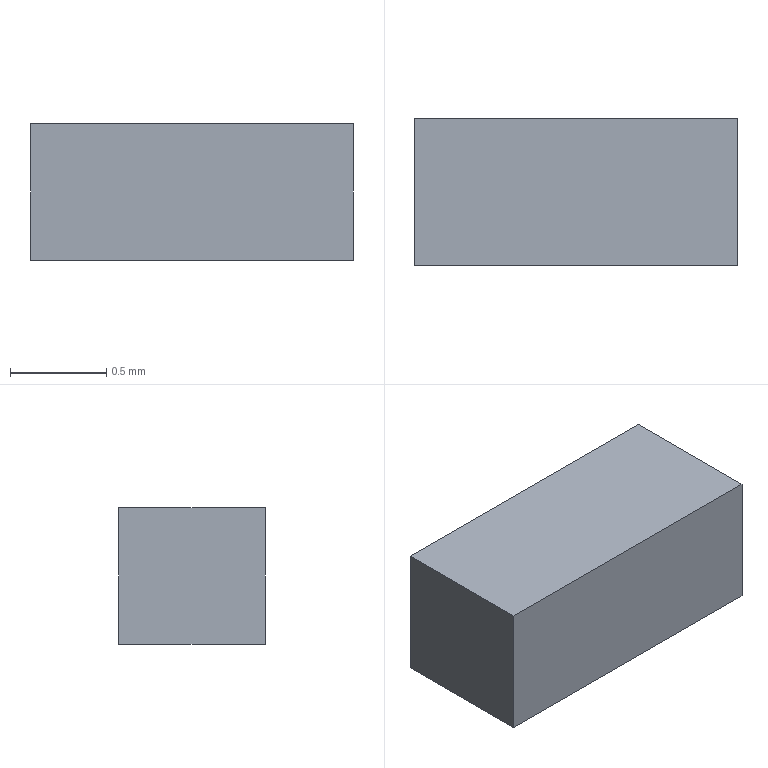Part | Creo | 1 solid | 6 faces | box 1.676 x 0.762 x 0.7099 mm | volume 0.9069 mm3 | plane 6
STEP:
#1=CARTESIAN_POINT('',(0.,0.,0.));
#2=DIRECTION('',(0.,0.,1.));
#3=DIRECTION('',(1.,0.,0.));
#4=AXIS2_PLACEMENT_3D('',#1,#2,#3);
#5=CARTESIAN_POINT('',(0.8384,-0.3809,0.));
#6=VERTEX_POINT('',#5);
#7=CARTESIAN_POINT('',(0.8384,0.3811,0.));
#8=VERTEX_POINT('',#7);
#9=CARTESIAN_POINT('',(0.8384,-0.3809,0.));
#10=DIRECTION('',(0.,1.,0.));
#11=VECTOR('',#10,0.762);
#12=LINE('',#9,#11);
#13=EDGE_CURVE('',#6,#8,#12,.T.);
#14=ORIENTED_EDGE('',*,*,#13,.T.);
#15=CARTESIAN_POINT('',(-0.838,0.3811,0.));
#16=VERTEX_POINT('',#15);
#17=CARTESIAN_POINT('',(0.8384,0.3811,0.));
#18=DIRECTION('',(-1.,0.,0.));
#19=VECTOR('',#18,1.676);
#20=LINE('',#17,#19);
#21=EDGE_CURVE('',#8,#16,#20,.T.);
#22=ORIENTED_EDGE('',*,*,#21,.T.);
#23=CARTESIAN_POINT('',(-0.838,-0.3809,0.));
#24=VERTEX_POINT('',#23);
#25=CARTESIAN_POINT('',(-0.838,0.3811,0.));
#26=DIRECTION('',(0.,-1.,0.));
#27=VECTOR('',#26,0.762);
#28=LINE('',#25,#27);
#29=EDGE_CURVE('',#16,#24,#28,.T.);
#30=ORIENTED_EDGE('',*,*,#29,.T.);
#31=CARTESIAN_POINT('',(-0.838,-0.3809,0.));
#32=DIRECTION('',(1.,0.,0.));
#33=VECTOR('',#32,1.676);
#34=LINE('',#31,#33);
#35=EDGE_CURVE('',#24,#6,#34,.T.);
#36=ORIENTED_EDGE('',*,*,#35,.T.);
#37=EDGE_LOOP('',(#14,#22,#30,#36));
#38=FACE_OUTER_BOUND('',#37,.F.);
#39=CARTESIAN_POINT('',(0.,0.,0.));
#40=DIRECTION('',(0.,0.,1.));
#41=DIRECTION('',(1.,0.,0.));
#42=AXIS2_PLACEMENT_3D('',#39,#40,#41);
#43=PLANE('',#42);
#44=ADVANCED_FACE('',(#38),#43,.F.);
#45=ORIENTED_EDGE('',*,*,#13,.F.);
#46=CARTESIAN_POINT('',(0.8384,-0.3809,0.7099));
#47=VERTEX_POINT('',#46);
#48=CARTESIAN_POINT('',(0.8384,-0.3809,0.));
#49=DIRECTION('',(0.,0.,1.));
#50=VECTOR('',#49,0.7099);
#51=LINE('',#48,#50);
#52=EDGE_CURVE('',#6,#47,#51,.T.);
#53=ORIENTED_EDGE('',*,*,#52,.T.);
#54=CARTESIAN_POINT('',(0.8384,0.3811,0.7099));
#55=VERTEX_POINT('',#54);
#56=CARTESIAN_POINT('',(0.8384,-0.3809,0.7099));
#57=DIRECTION('',(0.,1.,0.));
#58=VECTOR('',#57,0.762);
#59=LINE('',#56,#58);
#60=EDGE_CURVE('',#47,#55,#59,.T.);
#61=ORIENTED_EDGE('',*,*,#60,.T.);
#62=CARTESIAN_POINT('',(0.8384,0.3811,0.));
#63=DIRECTION('',(0.,0.,1.));
#64=VECTOR('',#63,0.7099);
#65=LINE('',#62,#64);
#66=EDGE_CURVE('',#8,#55,#65,.T.);
#67=ORIENTED_EDGE('',*,*,#66,.F.);
#68=EDGE_LOOP('',(#45,#53,#61,#67));
#69=FACE_OUTER_BOUND('',#68,.F.);
#70=CARTESIAN_POINT('',(0.8384,-0.3809,0.));
#71=DIRECTION('',(1.,0.,0.));
#72=DIRECTION('',(0.,1.,0.));
#73=AXIS2_PLACEMENT_3D('',#70,#71,#72);
#74=PLANE('',#73);
#75=ADVANCED_FACE('',(#69),#74,.T.);
#76=ORIENTED_EDGE('',*,*,#35,.F.);
#77=CARTESIAN_POINT('',(-0.838,-0.3809,0.7099));
#78=VERTEX_POINT('',#77);
#79=CARTESIAN_POINT('',(-0.838,-0.3809,0.));
#80=DIRECTION('',(0.,0.,1.));
#81=VECTOR('',#80,0.7099);
#82=LINE('',#79,#81);
#83=EDGE_CURVE('',#24,#78,#82,.T.);
#84=ORIENTED_EDGE('',*,*,#83,.T.);
#85=CARTESIAN_POINT('',(-0.838,-0.3809,0.7099));
#86=DIRECTION('',(1.,0.,0.));
#87=VECTOR('',#86,1.676);
#88=LINE('',#85,#87);
#89=EDGE_CURVE('',#78,#47,#88,.T.);
#90=ORIENTED_EDGE('',*,*,#89,.T.);
#91=ORIENTED_EDGE('',*,*,#52,.F.);
#92=EDGE_LOOP('',(#76,#84,#90,#91));
#93=FACE_OUTER_BOUND('',#92,.F.);
#94=CARTESIAN_POINT('',(-0.838,-0.3809,0.));
#95=DIRECTION('',(0.,-1.,0.));
#96=DIRECTION('',(1.,0.,0.));
#97=AXIS2_PLACEMENT_3D('',#94,#95,#96);
#98=PLANE('',#97);
#99=ADVANCED_FACE('',(#93),#98,.T.);
#100=ORIENTED_EDGE('',*,*,#29,.F.);
#101=CARTESIAN_POINT('',(-0.838,0.3811,0.7099));
#102=VERTEX_POINT('',#101);
#103=CARTESIAN_POINT('',(-0.838,0.3811,0.));
#104=DIRECTION('',(0.,0.,1.));
#105=VECTOR('',#104,0.7099);
#106=LINE('',#103,#105);
#107=EDGE_CURVE('',#16,#102,#106,.T.);
#108=ORIENTED_EDGE('',*,*,#107,.T.);
#109=CARTESIAN_POINT('',(-0.838,0.3811,0.7099));
#110=DIRECTION('',(0.,-1.,0.));
#111=VECTOR('',#110,0.762);
#112=LINE('',#109,#111);
#113=EDGE_CURVE('',#102,#78,#112,.T.);
#114=ORIENTED_EDGE('',*,*,#113,.T.);
#115=ORIENTED_EDGE('',*,*,#83,.F.);
#116=EDGE_LOOP('',(#100,#108,#114,#115));
#117=FACE_OUTER_BOUND('',#116,.F.);
#118=CARTESIAN_POINT('',(-0.838,0.3811,0.));
#119=DIRECTION('',(-1.,0.,0.));
#120=DIRECTION('',(0.,-1.,0.));
#121=AXIS2_PLACEMENT_3D('',#118,#119,#120);
#122=PLANE('',#121);
#123=ADVANCED_FACE('',(#117),#122,.T.);
#124=ORIENTED_EDGE('',*,*,#21,.F.);
#125=ORIENTED_EDGE('',*,*,#66,.T.);
#126=CARTESIAN_POINT('',(0.8384,0.3811,0.7099));
#127=DIRECTION('',(-1.,0.,0.));
#128=VECTOR('',#127,1.676);
#129=LINE('',#126,#128);
#130=EDGE_CURVE('',#55,#102,#129,.T.);
#131=ORIENTED_EDGE('',*,*,#130,.T.);
#132=ORIENTED_EDGE('',*,*,#107,.F.);
#133=EDGE_LOOP('',(#124,#125,#131,#132));
#134=FACE_OUTER_BOUND('',#133,.F.);
#135=CARTESIAN_POINT('',(0.8384,0.3811,0.));
#136=DIRECTION('',(0.,1.,0.));
#137=DIRECTION('',(-1.,0.,0.));
#138=AXIS2_PLACEMENT_3D('',#135,#136,#137);
#139=PLANE('',#138);
#140=ADVANCED_FACE('',(#134),#139,.T.);
#141=ORIENTED_EDGE('',*,*,#60,.F.);
#142=ORIENTED_EDGE('',*,*,#89,.F.);
#143=ORIENTED_EDGE('',*,*,#113,.F.);
#144=ORIENTED_EDGE('',*,*,#130,.F.);
#145=EDGE_LOOP('',(#141,#142,#143,#144));
#146=FACE_OUTER_BOUND('',#145,.F.);
#147=CARTESIAN_POINT('',(0.,0.,0.7099));
#148=DIRECTION('',(0.,0.,1.));
#149=DIRECTION('',(1.,0.,0.));
#150=AXIS2_PLACEMENT_3D('',#147,#148,#149);
#151=PLANE('',#150);
#152=ADVANCED_FACE('',(#146),#151,.T.);
#153=CLOSED_SHELL('',(#44,#75,#99,#123,#140,#152));
#154=MANIFOLD_SOLID_BREP('',#153);
#155=(LENGTH_UNIT()NAMED_UNIT(*)SI_UNIT(.MILLI.,.METRE.));
#156=UNCERTAINTY_MEASURE_WITH_UNIT(LENGTH_MEASURE(0.0001973),#155,'','');
#157=(NAMED_UNIT(*)PLANE_ANGLE_UNIT()SI_UNIT($,.RADIAN.));
#158=PLANE_ANGLE_MEASURE_WITH_UNIT(PLANE_ANGLE_MEASURE(0.01745),#157);
#159=(CONVERSION_BASED_UNIT('DEGREE',#158)NAMED_UNIT(*)PLANE_ANGLE_UNIT());
#160=(NAMED_UNIT(*)SI_UNIT($,.STERADIAN.)SOLID_ANGLE_UNIT());
#161=(GEOMETRIC_REPRESENTATION_CONTEXT(3)GLOBAL_UNCERTAINTY_ASSIGNED_CONTEXT((#156))GLOBAL_UNIT_ASSIGNED_CONTEXT((#155,#159,#160))REPRESENTATION_CONTEXT('',''));
#162=ADVANCED_BREP_SHAPE_REPRESENTATION('',(#4,#154),#161);